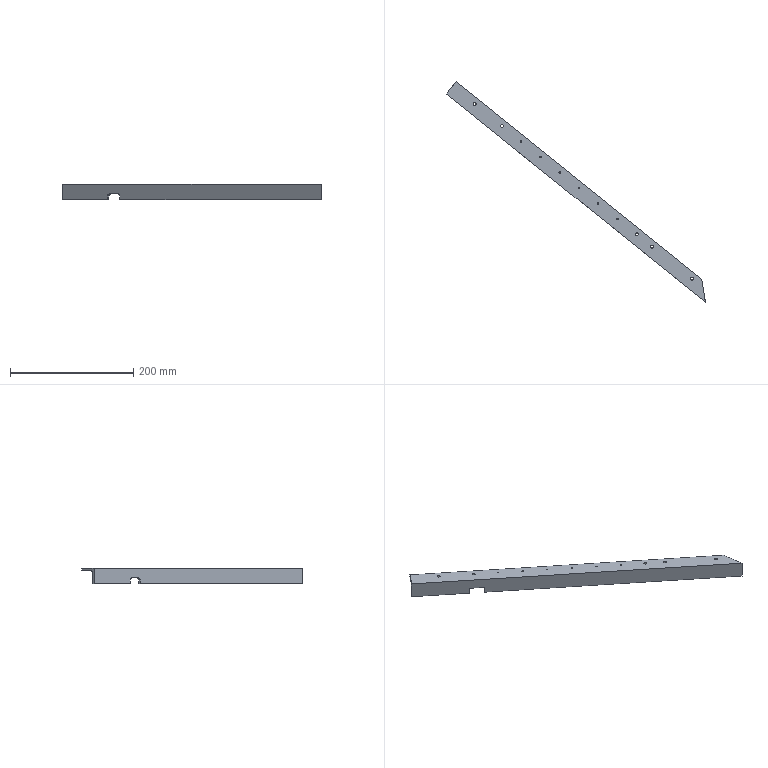Part | NX | features MG0301 nose pivot 24(right) 2 | 1 solid | 26 faces | box 419.376 x 356.955 x 25.4 mm | volume 81586 mm3 | cylinder 14 | plane 12 | commonest cylinder face diameters 2.4 x6 4.763 x5 6.35 x2 9.525 x1
STEP:
#1=CARTESIAN_POINT('',(357.102,-185.029,113.315));
#2=VERTEX_POINT('',#1);
#3=CARTESIAN_POINT('',(357.102,-185.029,106.965));
#4=VERTEX_POINT('',#3);
#5=CARTESIAN_POINT('',(357.102,-185.029,113.315));
#6=DIRECTION('',(0.,0.,-1.));
#7=VECTOR('',#6,1000.);
#8=LINE('',#5,#7);
#9=EDGE_CURVE('',#2,#4,#8,.T.);
#10=ORIENTED_EDGE('',*,*,#9,.F.);
#11=CARTESIAN_POINT('',(359.577,-187.018,116.49));
#12=VERTEX_POINT('',#11);
#13=CARTESIAN_POINT('',(359.577,-187.018,113.315));
#14=DIRECTION('',(-0.6266,-0.7794,0.));
#15=DIRECTION('',(0.7794,-0.6266,0.));
#16=AXIS2_PLACEMENT_3D('',#13,#14,#15);
#17=CIRCLE('',#16,3.175);
#18=EDGE_CURVE('',#12,#2,#17,.T.);
#19=ORIENTED_EDGE('',*,*,#18,.F.);
#20=CARTESIAN_POINT('',(374.424,-198.955,116.49));
#21=VERTEX_POINT('',#20);
#22=CARTESIAN_POINT('',(374.424,-198.955,116.49));
#23=DIRECTION('',(-0.7794,0.6266,0.));
#24=VECTOR('',#23,1000.);
#25=LINE('',#22,#24);
#26=EDGE_CURVE('',#21,#12,#25,.T.);
#27=ORIENTED_EDGE('',*,*,#26,.F.);
#28=CARTESIAN_POINT('',(376.898,-200.944,113.315));
#29=VERTEX_POINT('',#28);
#30=CARTESIAN_POINT('',(374.424,-198.955,113.315));
#31=DIRECTION('',(-0.6266,-0.7794,0.));
#32=DIRECTION('',(0.7794,-0.6266,0.));
#33=AXIS2_PLACEMENT_3D('',#30,#31,#32);
#34=CIRCLE('',#33,3.175);
#35=EDGE_CURVE('',#29,#21,#34,.T.);
#36=ORIENTED_EDGE('',*,*,#35,.F.);
#37=CARTESIAN_POINT('',(376.898,-200.944,106.965));
#38=VERTEX_POINT('',#37);
#39=CARTESIAN_POINT('',(376.898,-200.944,106.965));
#40=DIRECTION('',(0.,0.,1.));
#41=VECTOR('',#40,1000.);
#42=LINE('',#39,#41);
#43=EDGE_CURVE('',#38,#29,#42,.T.);
#44=ORIENTED_EDGE('',*,*,#43,.F.);
#45=CARTESIAN_POINT('',(703.42,-463.453,106.965));
#46=VERTEX_POINT('',#45);
#47=CARTESIAN_POINT('',(284.044,-126.294,106.965));
#48=DIRECTION('',(0.7794,-0.6266,0.));
#49=VECTOR('',#48,1000.);
#50=LINE('',#47,#49);
#51=EDGE_CURVE('',#46,#38,#50,.F.);
#52=ORIENTED_EDGE('',*,*,#51,.F.);
#53=CARTESIAN_POINT('',(703.42,-463.453,132.365));
#54=VERTEX_POINT('',#53);
#55=CARTESIAN_POINT('',(703.42,-463.453,132.365));
#56=DIRECTION('',(0.,0.,1.));
#57=VECTOR('',#56,1000.);
#58=LINE('',#55,#57);
#59=EDGE_CURVE('',#54,#46,#58,.F.);
#60=ORIENTED_EDGE('',*,*,#59,.F.);
#61=CARTESIAN_POINT('',(284.044,-126.294,132.365));
#62=VERTEX_POINT('',#61);
#63=CARTESIAN_POINT('',(284.044,-126.294,132.365));
#64=DIRECTION('',(0.7794,-0.6266,0.));
#65=VECTOR('',#64,1000.);
#66=LINE('',#63,#65);
#67=EDGE_CURVE('',#54,#62,#66,.F.);
#68=ORIENTED_EDGE('',*,*,#67,.T.);
#69=CARTESIAN_POINT('',(284.044,-126.294,106.965));
#70=VERTEX_POINT('',#69);
#71=CARTESIAN_POINT('',(284.044,-126.294,132.365));
#72=DIRECTION('',(0.,0.,1.));
#73=VECTOR('',#72,1000.);
#74=LINE('',#71,#73);
#75=EDGE_CURVE('',#62,#70,#74,.F.);
#76=ORIENTED_EDGE('',*,*,#75,.T.);
#77=CARTESIAN_POINT('',(284.044,-126.294,106.965));
#78=DIRECTION('',(0.7794,-0.6266,0.));
#79=VECTOR('',#78,1000.);
#80=LINE('',#77,#79);
#81=EDGE_CURVE('',#4,#70,#80,.F.);
#82=ORIENTED_EDGE('',*,*,#81,.F.);
#83=EDGE_LOOP('',(#10,#19,#27,#36,#44,#52,#60,#68,#76,#82));
#84=FACE_BOUND('',#83,.T.);
#85=CARTESIAN_POINT('',(284.044,-126.294,132.365));
#86=DIRECTION('',(0.6266,0.7794,0.));
#87=DIRECTION('',(-0.7794,0.6266,0.));
#88=AXIS2_PLACEMENT_3D('',#85,#86,#87);
#89=PLANE('',#88);
#90=ADVANCED_FACE('',(#84),#89,.F.);
#91=CARTESIAN_POINT('',(378.888,-198.469,106.965));
#92=VERTEX_POINT('',#91);
#93=CARTESIAN_POINT('',(383.164,-193.15,106.965));
#94=DIRECTION('',(-0.6266,-0.7794,0.));
#95=VECTOR('',#94,1000.);
#96=LINE('',#93,#95);
#97=EDGE_CURVE('',#92,#38,#96,.T.);
#98=ORIENTED_EDGE('',*,*,#97,.F.);
#99=CARTESIAN_POINT('',(702.681,-458.785,106.965));
#100=VERTEX_POINT('',#99);
#101=CARTESIAN_POINT('',(286.034,-123.819,106.965));
#102=DIRECTION('',(0.7794,-0.6266,0.));
#103=VECTOR('',#102,1000.);
#104=LINE('',#101,#103);
#105=EDGE_CURVE('',#100,#92,#104,.F.);
#106=ORIENTED_EDGE('',*,*,#105,.F.);
#107=CARTESIAN_POINT('',(641.063,-69.747,106.965));
#108=DIRECTION('',(0.1564,-0.9877,0.));
#109=VECTOR('',#108,1000.);
#110=LINE('',#107,#109);
#111=EDGE_CURVE('',#46,#100,#110,.F.);
#112=ORIENTED_EDGE('',*,*,#111,.F.);
#113=ORIENTED_EDGE('',*,*,#51,.T.);
#114=EDGE_LOOP('',(#98,#106,#112,#113));
#115=FACE_BOUND('',#114,.T.);
#116=CARTESIAN_POINT('',(284.044,-126.294,106.965));
#117=DIRECTION('',(0.,0.,1.));
#118=DIRECTION('',(0.9931,0.1177,0.));
#119=AXIS2_PLACEMENT_3D('',#116,#117,#118);
#120=PLANE('',#119);
#121=ADVANCED_FACE('',(#115),#120,.F.);
#122=CARTESIAN_POINT('',(437.141,-229.007,129.19));
#123=VERTEX_POINT('',#122);
#124=CARTESIAN_POINT('',(436.205,-228.255,129.19));
#125=DIRECTION('',(0.,0.,1.));
#126=DIRECTION('',(0.7794,-0.6266,0.));
#127=AXIS2_PLACEMENT_3D('',#124,#125,#126);
#128=CIRCLE('',#127,1.2);
#129=EDGE_CURVE('',#123,#123,#128,.F.);
#130=ORIENTED_EDGE('',*,*,#129,.F.);
#131=EDGE_LOOP('',(#130));
#132=FACE_BOUND('',#131,.T.);
#133=CARTESIAN_POINT('',(499.49,-279.133,129.19));
#134=VERTEX_POINT('',#133);
#135=CARTESIAN_POINT('',(498.554,-278.381,129.19));
#136=DIRECTION('',(0.,0.,1.));
#137=DIRECTION('',(0.7794,-0.6266,0.));
#138=AXIS2_PLACEMENT_3D('',#135,#136,#137);
#139=CIRCLE('',#138,1.2);
#140=EDGE_CURVE('',#134,#134,#139,.F.);
#141=ORIENTED_EDGE('',*,*,#140,.F.);
#142=EDGE_LOOP('',(#141));
#143=FACE_BOUND('',#142,.T.);
#144=CARTESIAN_POINT('',(561.839,-329.259,129.19));
#145=VERTEX_POINT('',#144);
#146=CARTESIAN_POINT('',(560.903,-328.507,129.19));
#147=DIRECTION('',(0.,0.,1.));
#148=DIRECTION('',(0.7794,-0.6266,0.));
#149=AXIS2_PLACEMENT_3D('',#146,#147,#148);
#150=CIRCLE('',#149,1.2);
#151=EDGE_CURVE('',#145,#145,#150,.F.);
#152=ORIENTED_EDGE('',*,*,#151,.F.);
#153=EDGE_LOOP('',(#152));
#154=FACE_BOUND('',#153,.T.);
#155=CARTESIAN_POINT('',(376.221,-177.849,129.19));
#156=VERTEX_POINT('',#155);
#157=CARTESIAN_POINT('',(373.856,-178.129,129.19));
#158=DIRECTION('',(0.,0.,1.));
#159=DIRECTION('',(0.9931,0.1177,0.));
#160=AXIS2_PLACEMENT_3D('',#157,#158,#159);
#161=CIRCLE('',#160,2.381);
#162=EDGE_CURVE('',#156,#156,#161,.F.);
#163=ORIENTED_EDGE('',*,*,#162,.F.);
#164=EDGE_LOOP('',(#163));
#165=FACE_BOUND('',#164,.T.);
#166=CARTESIAN_POINT('',(331.889,-142.208,129.19));
#167=VERTEX_POINT('',#166);
#168=CARTESIAN_POINT('',(329.524,-142.488,129.19));
#169=DIRECTION('',(0.,0.,1.));
#170=DIRECTION('',(0.9931,0.1177,0.));
#171=AXIS2_PLACEMENT_3D('',#168,#169,#170);
#172=CIRCLE('',#171,2.381);
#173=EDGE_CURVE('',#167,#167,#172,.F.);
#174=ORIENTED_EDGE('',*,*,#173,.F.);
#175=EDGE_LOOP('',(#174));
#176=FACE_BOUND('',#175,.T.);
#177=CARTESIAN_POINT('',(619.193,-373.188,129.19));
#178=VERTEX_POINT('',#177);
#179=CARTESIAN_POINT('',(616.829,-373.468,129.19));
#180=DIRECTION('',(0.,0.,1.));
#181=DIRECTION('',(0.9931,0.1177,0.));
#182=AXIS2_PLACEMENT_3D('',#179,#180,#181);
#183=CIRCLE('',#182,2.381);
#184=EDGE_CURVE('',#178,#178,#183,.F.);
#185=ORIENTED_EDGE('',*,*,#184,.F.);
#186=EDGE_LOOP('',(#185));
#187=FACE_BOUND('',#186,.T.);
#188=CARTESIAN_POINT('',(594.449,-353.294,129.19));
#189=VERTEX_POINT('',#188);
#190=CARTESIAN_POINT('',(592.084,-353.574,129.19));
#191=DIRECTION('',(0.,0.,1.));
#192=DIRECTION('',(0.9931,0.1177,0.));
#193=AXIS2_PLACEMENT_3D('',#190,#191,#192);
#194=CIRCLE('',#193,2.381);
#195=EDGE_CURVE('',#189,#189,#194,.F.);
#196=ORIENTED_EDGE('',*,*,#195,.F.);
#197=EDGE_LOOP('',(#196));
#198=FACE_BOUND('',#197,.T.);
#199=CARTESIAN_POINT('',(683.67,-425.024,129.19));
#200=VERTEX_POINT('',#199);
#201=CARTESIAN_POINT('',(681.305,-425.304,129.19));
#202=DIRECTION('',(0.,0.,1.));
#203=DIRECTION('',(0.9931,0.1177,0.));
#204=AXIS2_PLACEMENT_3D('',#201,#202,#203);
#205=CIRCLE('',#204,2.381);
#206=EDGE_CURVE('',#200,#200,#205,.F.);
#207=ORIENTED_EDGE('',*,*,#206,.F.);
#208=EDGE_LOOP('',(#207));
#209=FACE_BOUND('',#208,.T.);
#210=CARTESIAN_POINT('',(697.505,-426.107,129.19));
#211=VERTEX_POINT('',#210);
#212=CARTESIAN_POINT('',(299.959,-106.498,129.19));
#213=VERTEX_POINT('',#212);
#214=CARTESIAN_POINT('',(299.959,-106.498,129.19));
#215=DIRECTION('',(0.7794,-0.6266,0.));
#216=VECTOR('',#215,1000.);
#217=LINE('',#214,#216);
#218=EDGE_CURVE('',#211,#213,#217,.F.);
#219=ORIENTED_EDGE('',*,*,#218,.F.);
#220=CARTESIAN_POINT('',(701.572,-451.782,129.19));
#221=VERTEX_POINT('',#220);
#222=CARTESIAN_POINT('',(638.394,-52.895,129.19));
#223=DIRECTION('',(0.1564,-0.9877,0.));
#224=VECTOR('',#223,1000.);
#225=LINE('',#222,#224);
#226=EDGE_CURVE('',#221,#211,#225,.F.);
#227=ORIENTED_EDGE('',*,*,#226,.F.);
#228=CARTESIAN_POINT('',(289.018,-120.107,129.19));
#229=VERTEX_POINT('',#228);
#230=CARTESIAN_POINT('',(289.018,-120.107,129.19));
#231=DIRECTION('',(0.7794,-0.6266,0.));
#232=VECTOR('',#231,1000.);
#233=LINE('',#230,#232);
#234=EDGE_CURVE('',#221,#229,#233,.F.);
#235=ORIENTED_EDGE('',*,*,#234,.T.);
#236=CARTESIAN_POINT('',(299.959,-106.498,129.19));
#237=DIRECTION('',(-0.6266,-0.7794,0.));
#238=VECTOR('',#237,1000.);
#239=LINE('',#236,#238);
#240=EDGE_CURVE('',#229,#213,#239,.F.);
#241=ORIENTED_EDGE('',*,*,#240,.T.);
#242=EDGE_LOOP('',(#219,#227,#235,#241));
#243=FACE_BOUND('',#242,.T.);
#244=CARTESIAN_POINT('',(530.664,-304.196,129.19));
#245=VERTEX_POINT('',#244);
#246=CARTESIAN_POINT('',(529.729,-303.444,129.19));
#247=DIRECTION('',(0.,0.,1.));
#248=DIRECTION('',(0.7794,-0.6266,0.));
#249=AXIS2_PLACEMENT_3D('',#246,#247,#248);
#250=CIRCLE('',#249,1.2);
#251=EDGE_CURVE('',#245,#245,#250,.F.);
#252=ORIENTED_EDGE('',*,*,#251,.F.);
#253=EDGE_LOOP('',(#252));
#254=FACE_BOUND('',#253,.T.);
#255=CARTESIAN_POINT('',(468.315,-254.07,129.19));
#256=VERTEX_POINT('',#255);
#257=CARTESIAN_POINT('',(467.38,-253.318,129.19));
#258=DIRECTION('',(0.,0.,1.));
#259=DIRECTION('',(0.7794,-0.6266,0.));
#260=AXIS2_PLACEMENT_3D('',#257,#258,#259);
#261=CIRCLE('',#260,1.2);
#262=EDGE_CURVE('',#256,#256,#261,.F.);
#263=ORIENTED_EDGE('',*,*,#262,.F.);
#264=EDGE_LOOP('',(#263));
#265=FACE_BOUND('',#264,.T.);
#266=CARTESIAN_POINT('',(405.966,-203.944,129.19));
#267=VERTEX_POINT('',#266);
#268=CARTESIAN_POINT('',(405.031,-203.192,129.19));
#269=DIRECTION('',(0.,0.,1.));
#270=DIRECTION('',(0.7794,-0.6266,0.));
#271=AXIS2_PLACEMENT_3D('',#268,#269,#270);
#272=CIRCLE('',#271,1.2);
#273=EDGE_CURVE('',#267,#267,#272,.F.);
#274=ORIENTED_EDGE('',*,*,#273,.F.);
#275=EDGE_LOOP('',(#274));
#276=FACE_BOUND('',#275,.T.);
#277=CARTESIAN_POINT('',(299.959,-106.498,129.19));
#278=DIRECTION('',(0.,0.,1.));
#279=DIRECTION('',(0.9931,0.1177,0.));
#280=AXIS2_PLACEMENT_3D('',#277,#278,#279);
#281=PLANE('',#280);
#282=ADVANCED_FACE('',(#132,#143,#154,#165,#176,#187,#198,#209,#243,#254,#265,#276),#281,.F.);
#283=CARTESIAN_POINT('',(406.222,-203.051,132.365));
#284=VERTEX_POINT('',#283);
#285=CARTESIAN_POINT('',(405.031,-203.192,132.365));
#286=DIRECTION('',(0.,0.,1.));
#287=DIRECTION('',(0.9931,0.1177,0.));
#288=AXIS2_PLACEMENT_3D('',#285,#286,#287);
#289=CIRCLE('',#288,1.2);
#290=EDGE_CURVE('',#284,#284,#289,.F.);
#291=ORIENTED_EDGE('',*,*,#290,.T.);
#292=EDGE_LOOP('',(#291));
#293=FACE_BOUND('',#292,.T.);
#294=CARTESIAN_POINT('',(437.397,-228.114,132.365));
#295=VERTEX_POINT('',#294);
#296=CARTESIAN_POINT('',(436.205,-228.255,132.365));
#297=DIRECTION('',(0.,0.,1.));
#298=DIRECTION('',(0.9931,0.1177,0.));
#299=AXIS2_PLACEMENT_3D('',#296,#297,#298);
#300=CIRCLE('',#299,1.2);
#301=EDGE_CURVE('',#295,#295,#300,.F.);
#302=ORIENTED_EDGE('',*,*,#301,.T.);
#303=EDGE_LOOP('',(#302));
#304=FACE_BOUND('',#303,.T.);
#305=CARTESIAN_POINT('',(468.572,-253.177,132.365));
#306=VERTEX_POINT('',#305);
#307=CARTESIAN_POINT('',(467.38,-253.318,132.365));
#308=DIRECTION('',(0.,0.,1.));
#309=DIRECTION('',(0.9931,0.1177,0.));
#310=AXIS2_PLACEMENT_3D('',#307,#308,#309);
#311=CIRCLE('',#310,1.2);
#312=EDGE_CURVE('',#306,#306,#311,.F.);
#313=ORIENTED_EDGE('',*,*,#312,.T.);
#314=EDGE_LOOP('',(#313));
#315=FACE_BOUND('',#314,.T.);
#316=CARTESIAN_POINT('',(499.746,-278.24,132.365));
#317=VERTEX_POINT('',#316);
#318=CARTESIAN_POINT('',(498.554,-278.381,132.365));
#319=DIRECTION('',(0.,0.,1.));
#320=DIRECTION('',(0.9931,0.1177,0.));
#321=AXIS2_PLACEMENT_3D('',#318,#319,#320);
#322=CIRCLE('',#321,1.2);
#323=EDGE_CURVE('',#317,#317,#322,.F.);
#324=ORIENTED_EDGE('',*,*,#323,.T.);
#325=EDGE_LOOP('',(#324));
#326=FACE_BOUND('',#325,.T.);
#327=CARTESIAN_POINT('',(530.921,-303.303,132.365));
#328=VERTEX_POINT('',#327);
#329=CARTESIAN_POINT('',(529.729,-303.444,132.365));
#330=DIRECTION('',(0.,0.,1.));
#331=DIRECTION('',(0.9931,0.1177,0.));
#332=AXIS2_PLACEMENT_3D('',#329,#330,#331);
#333=CIRCLE('',#332,1.2);
#334=EDGE_CURVE('',#328,#328,#333,.F.);
#335=ORIENTED_EDGE('',*,*,#334,.T.);
#336=EDGE_LOOP('',(#335));
#337=FACE_BOUND('',#336,.T.);
#338=CARTESIAN_POINT('',(562.095,-328.365,132.365));
#339=VERTEX_POINT('',#338);
#340=CARTESIAN_POINT('',(560.903,-328.507,132.365));
#341=DIRECTION('',(0.,0.,1.));
#342=DIRECTION('',(0.9931,0.1177,0.));
#343=AXIS2_PLACEMENT_3D('',#340,#341,#342);
#344=CIRCLE('',#343,1.2);
#345=EDGE_CURVE('',#339,#339,#344,.F.);
#346=ORIENTED_EDGE('',*,*,#345,.T.);
#347=EDGE_LOOP('',(#346));
#348=FACE_BOUND('',#347,.T.);
#349=CARTESIAN_POINT('',(376.221,-177.849,132.365));
#350=VERTEX_POINT('',#349);
#351=CARTESIAN_POINT('',(373.856,-178.129,132.365));
#352=DIRECTION('',(0.,0.,1.));
#353=DIRECTION('',(0.9931,0.1177,0.));
#354=AXIS2_PLACEMENT_3D('',#351,#352,#353);
#355=CIRCLE('',#354,2.381);
#356=EDGE_CURVE('',#350,#350,#355,.F.);
#357=ORIENTED_EDGE('',*,*,#356,.T.);
#358=EDGE_LOOP('',(#357));
#359=FACE_BOUND('',#358,.T.);
#360=CARTESIAN_POINT('',(331.889,-142.208,132.365));
#361=VERTEX_POINT('',#360);
#362=CARTESIAN_POINT('',(329.524,-142.488,132.365));
#363=DIRECTION('',(0.,0.,1.));
#364=DIRECTION('',(0.9931,0.1177,0.));
#365=AXIS2_PLACEMENT_3D('',#362,#363,#364);
#366=CIRCLE('',#365,2.381);
#367=EDGE_CURVE('',#361,#361,#366,.F.);
#368=ORIENTED_EDGE('',*,*,#367,.T.);
#369=EDGE_LOOP('',(#368));
#370=FACE_BOUND('',#369,.T.);
#371=CARTESIAN_POINT('',(619.193,-373.188,132.365));
#372=VERTEX_POINT('',#371);
#373=CARTESIAN_POINT('',(616.829,-373.468,132.365));
#374=DIRECTION('',(0.,0.,1.));
#375=DIRECTION('',(0.9931,0.1177,0.));
#376=AXIS2_PLACEMENT_3D('',#373,#374,#375);
#377=CIRCLE('',#376,2.381);
#378=EDGE_CURVE('',#372,#372,#377,.F.);
#379=ORIENTED_EDGE('',*,*,#378,.T.);
#380=EDGE_LOOP('',(#379));
#381=FACE_BOUND('',#380,.T.);
#382=CARTESIAN_POINT('',(594.449,-353.294,132.365));
#383=VERTEX_POINT('',#382);
#384=CARTESIAN_POINT('',(592.084,-353.574,132.365));
#385=DIRECTION('',(0.,0.,1.));
#386=DIRECTION('',(0.9931,0.1177,0.));
#387=AXIS2_PLACEMENT_3D('',#384,#385,#386);
#388=CIRCLE('',#387,2.381);
#389=EDGE_CURVE('',#383,#383,#388,.F.);
#390=ORIENTED_EDGE('',*,*,#389,.T.);
#391=EDGE_LOOP('',(#390));
#392=FACE_BOUND('',#391,.T.);
#393=CARTESIAN_POINT('',(683.67,-425.024,132.365));
#394=VERTEX_POINT('',#393);
#395=CARTESIAN_POINT('',(681.305,-425.304,132.365));
#396=DIRECTION('',(0.,0.,1.));
#397=DIRECTION('',(0.9931,0.1177,0.));
#398=AXIS2_PLACEMENT_3D('',#395,#396,#397);
#399=CIRCLE('',#398,2.381);
#400=EDGE_CURVE('',#394,#394,#399,.F.);
#401=ORIENTED_EDGE('',*,*,#400,.T.);
#402=EDGE_LOOP('',(#401));
#403=FACE_BOUND('',#402,.T.);
#404=ORIENTED_EDGE('',*,*,#67,.F.);
#405=CARTESIAN_POINT('',(697.505,-426.107,132.365));
#406=VERTEX_POINT('',#405);
#407=CARTESIAN_POINT('',(641.063,-69.747,132.365));
#408=DIRECTION('',(-0.1564,0.9877,0.));
#409=VECTOR('',#408,1000.);
#410=LINE('',#407,#409);
#411=EDGE_CURVE('',#406,#54,#410,.F.);
#412=ORIENTED_EDGE('',*,*,#411,.F.);
#413=CARTESIAN_POINT('',(299.959,-106.498,132.365));
#414=VERTEX_POINT('',#413);
#415=CARTESIAN_POINT('',(299.959,-106.498,132.365));
#416=DIRECTION('',(0.7794,-0.6266,0.));
#417=VECTOR('',#416,1000.);
#418=LINE('',#415,#417);
#419=EDGE_CURVE('',#406,#414,#418,.F.);
#420=ORIENTED_EDGE('',*,*,#419,.T.);
#421=CARTESIAN_POINT('',(284.044,-126.294,132.365));
#422=DIRECTION('',(0.6266,0.7794,0.));
#423=VECTOR('',#422,1000.);
#424=LINE('',#421,#423);
#425=EDGE_CURVE('',#414,#62,#424,.F.);
#426=ORIENTED_EDGE('',*,*,#425,.T.);
#427=EDGE_LOOP('',(#404,#412,#420,#426));
#428=FACE_BOUND('',#427,.T.);
#429=CARTESIAN_POINT('',(284.044,-126.294,132.365));
#430=DIRECTION('',(0.,0.,-1.));
#431=DIRECTION('',(-0.9931,-0.1177,0.));
#432=AXIS2_PLACEMENT_3D('',#429,#430,#431);
#433=PLANE('',#432);
#434=ADVANCED_FACE('',(#293,#304,#315,#326,#337,#348,#359,#370,#381,#392,#403,#428),#433,.F.);
#435=ORIENTED_EDGE('',*,*,#419,.F.);
#436=CARTESIAN_POINT('',(697.505,-426.107,132.365));
#437=DIRECTION('',(0.,0.,-1.));
#438=VECTOR('',#437,1000.);
#439=LINE('',#436,#438);
#440=EDGE_CURVE('',#211,#406,#439,.F.);
#441=ORIENTED_EDGE('',*,*,#440,.F.);
#442=ORIENTED_EDGE('',*,*,#218,.T.);
#443=CARTESIAN_POINT('',(299.959,-106.498,132.365));
#444=DIRECTION('',(0.,0.,-1.));
#445=VECTOR('',#444,1000.);
#446=LINE('',#443,#445);
#447=EDGE_CURVE('',#213,#414,#446,.F.);
#448=ORIENTED_EDGE('',*,*,#447,.T.);
#449=EDGE_LOOP('',(#435,#441,#442,#448));
#450=FACE_BOUND('',#449,.T.);
#451=CARTESIAN_POINT('',(299.959,-106.498,132.365));
#452=DIRECTION('',(-0.6266,-0.7794,0.));
#453=DIRECTION('',(0.7794,-0.6266,0.));
#454=AXIS2_PLACEMENT_3D('',#451,#452,#453);
#455=PLANE('',#454);
#456=ADVANCED_FACE('',(#450),#455,.F.);
#457=ORIENTED_EDGE('',*,*,#234,.F.);
#458=CARTESIAN_POINT('',(702.681,-458.785,124.427));
#459=VERTEX_POINT('',#458);
#460=CARTESIAN_POINT('',(701.572,-451.782,124.427));
#461=DIRECTION('',(-0.9877,-0.1564,0.));
#462=DIRECTION('',(0.1564,-0.9877,0.));
#463=AXIS2_PLACEMENT_3D('',#460,#461,#462);
#464=ELLIPSE('',#463,7.09,4.763);
#465=EDGE_CURVE('',#459,#221,#464,.T.);
#466=ORIENTED_EDGE('',*,*,#465,.F.);
#467=CARTESIAN_POINT('',(286.034,-123.819,124.427));
#468=VERTEX_POINT('',#467);
#469=CARTESIAN_POINT('',(286.034,-123.819,124.427));
#470=DIRECTION('',(0.7794,-0.6266,0.));
#471=VECTOR('',#470,1000.);
#472=LINE('',#469,#471);
#473=EDGE_CURVE('',#459,#468,#472,.F.);
#474=ORIENTED_EDGE('',*,*,#473,.T.);
#475=CARTESIAN_POINT('',(289.018,-120.107,124.427));
#476=DIRECTION('',(0.7794,-0.6266,0.));
#477=DIRECTION('',(-0.6266,-0.7794,0.));
#478=AXIS2_PLACEMENT_3D('',#475,#476,#477);
#479=CIRCLE('',#478,4.763);
#480=EDGE_CURVE('',#468,#229,#479,.F.);
#481=ORIENTED_EDGE('',*,*,#480,.T.);
#482=EDGE_LOOP('',(#457,#466,#474,#481));
#483=FACE_BOUND('',#482,.T.);
#484=CARTESIAN_POINT('',(289.018,-120.107,124.427));
#485=DIRECTION('',(0.7794,-0.6266,0.));
#486=DIRECTION('',(0.6266,0.7794,0.));
#487=AXIS2_PLACEMENT_3D('',#484,#485,#486);
#488=CYLINDRICAL_SURFACE('',#487,4.763);
#489=ADVANCED_FACE('',(#483),#488,.F.);
#490=CARTESIAN_POINT('',(361.566,-184.544,116.49));
#491=VERTEX_POINT('',#490);
#492=CARTESIAN_POINT('',(359.092,-182.555,113.315));
#493=VERTEX_POINT('',#492);
#494=CARTESIAN_POINT('',(361.566,-184.544,113.315));
#495=DIRECTION('',(-0.6266,-0.7794,0.));
#496=DIRECTION('',(0.7794,-0.6266,0.));
#497=AXIS2_PLACEMENT_3D('',#494,#495,#496);
#498=CIRCLE('',#497,3.175);
#499=EDGE_CURVE('',#491,#493,#498,.T.);
#500=ORIENTED_EDGE('',*,*,#499,.T.);
#501=CARTESIAN_POINT('',(359.092,-182.555,106.965));
#502=VERTEX_POINT('',#501);
#503=CARTESIAN_POINT('',(359.092,-182.555,106.965));
#504=DIRECTION('',(0.,0.,-1.));
#505=VECTOR('',#504,1000.);
#506=LINE('',#503,#505);
#507=EDGE_CURVE('',#493,#502,#506,.T.);
#508=ORIENTED_EDGE('',*,*,#507,.T.);
#509=CARTESIAN_POINT('',(286.034,-123.819,106.965));
#510=VERTEX_POINT('',#509);
#511=CARTESIAN_POINT('',(286.034,-123.819,106.965));
#512=DIRECTION('',(0.7794,-0.6266,0.));
#513=VECTOR('',#512,1000.);
#514=LINE('',#511,#513);
#515=EDGE_CURVE('',#502,#510,#514,.F.);
#516=ORIENTED_EDGE('',*,*,#515,.T.);
#517=CARTESIAN_POINT('',(286.034,-123.819,106.965));
#518=DIRECTION('',(0.,0.,-1.));
#519=VECTOR('',#518,1000.);
#520=LINE('',#517,#519);
#521=EDGE_CURVE('',#510,#468,#520,.F.);
#522=ORIENTED_EDGE('',*,*,#521,.T.);
#523=ORIENTED_EDGE('',*,*,#473,.F.);
#524=CARTESIAN_POINT('',(702.681,-458.785,106.965));
#525=DIRECTION('',(0.,0.,-1.));
#526=VECTOR('',#525,1000.);
#527=LINE('',#524,#526);
#528=EDGE_CURVE('',#100,#459,#527,.F.);
#529=ORIENTED_EDGE('',*,*,#528,.F.);
#530=ORIENTED_EDGE('',*,*,#105,.T.);
#531=CARTESIAN_POINT('',(378.888,-198.469,113.315));
#532=VERTEX_POINT('',#531);
#533=CARTESIAN_POINT('',(378.888,-198.469,106.965));
#534=DIRECTION('',(0.,0.,1.));
#535=VECTOR('',#534,1000.);
#536=LINE('',#533,#535);
#537=EDGE_CURVE('',#92,#532,#536,.T.);
#538=ORIENTED_EDGE('',*,*,#537,.T.);
#539=CARTESIAN_POINT('',(376.413,-196.48,116.49));
#540=VERTEX_POINT('',#539);
#541=CARTESIAN_POINT('',(376.413,-196.48,113.315));
#542=DIRECTION('',(-0.6266,-0.7794,0.));
#543=DIRECTION('',(0.7794,-0.6266,0.));
#544=AXIS2_PLACEMENT_3D('',#541,#542,#543);
#545=CIRCLE('',#544,3.175);
#546=EDGE_CURVE('',#532,#540,#545,.T.);
#547=ORIENTED_EDGE('',*,*,#546,.T.);
#548=CARTESIAN_POINT('',(286.034,-123.819,116.49));
#549=DIRECTION('',(-0.7794,0.6266,0.));
#550=VECTOR('',#549,1000.);
#551=LINE('',#548,#550);
#552=EDGE_CURVE('',#540,#491,#551,.T.);
#553=ORIENTED_EDGE('',*,*,#552,.T.);
#554=EDGE_LOOP('',(#500,#508,#516,#522,#523,#529,#530,#538,#547,#553));
#555=FACE_BOUND('',#554,.T.);
#556=CARTESIAN_POINT('',(286.034,-123.819,106.965));
#557=DIRECTION('',(-0.6266,-0.7794,0.));
#558=DIRECTION('',(0.7794,-0.6266,0.));
#559=AXIS2_PLACEMENT_3D('',#556,#557,#558);
#560=PLANE('',#559);
#561=ADVANCED_FACE('',(#555),#560,.F.);
#562=ORIENTED_EDGE('',*,*,#515,.F.);
#563=CARTESIAN_POINT('',(363.368,-177.235,106.965));
#564=DIRECTION('',(-0.6266,-0.7794,0.));
#565=VECTOR('',#564,1000.);
#566=LINE('',#563,#565);
#567=EDGE_CURVE('',#502,#4,#566,.T.);
#568=ORIENTED_EDGE('',*,*,#567,.T.);
#569=ORIENTED_EDGE('',*,*,#81,.T.);
#570=CARTESIAN_POINT('',(284.044,-126.294,106.965));
#571=DIRECTION('',(-0.6266,-0.7794,0.));
#572=VECTOR('',#571,1000.);
#573=LINE('',#570,#572);
#574=EDGE_CURVE('',#70,#510,#573,.F.);
#575=ORIENTED_EDGE('',*,*,#574,.T.);
#576=EDGE_LOOP('',(#562,#568,#569,#575));
#577=FACE_BOUND('',#576,.T.);
#578=CARTESIAN_POINT('',(284.044,-126.294,106.965));
#579=DIRECTION('',(0.,0.,1.));
#580=DIRECTION('',(0.9931,0.1177,0.));
#581=AXIS2_PLACEMENT_3D('',#578,#579,#580);
#582=PLANE('',#581);
#583=ADVANCED_FACE('',(#577),#582,.F.);
#584=ORIENTED_EDGE('',*,*,#75,.F.);
#585=ORIENTED_EDGE('',*,*,#425,.F.);
#586=ORIENTED_EDGE('',*,*,#447,.F.);
#587=ORIENTED_EDGE('',*,*,#240,.F.);
#588=ORIENTED_EDGE('',*,*,#480,.F.);
#589=ORIENTED_EDGE('',*,*,#521,.F.);
#590=ORIENTED_EDGE('',*,*,#574,.F.);
#591=EDGE_LOOP('',(#584,#585,#586,#587,#588,#589,#590));
#592=FACE_BOUND('',#591,.T.);
#593=CARTESIAN_POINT('',(289.018,-120.107,124.427));
#594=DIRECTION('',(-0.7794,0.6266,0.));
#595=DIRECTION('',(-0.6266,-0.7794,0.));
#596=AXIS2_PLACEMENT_3D('',#593,#594,#595);
#597=PLANE('',#596);
#598=ADVANCED_FACE('',(#592),#597,.T.);
#599=ORIENTED_EDGE('',*,*,#411,.T.);
#600=ORIENTED_EDGE('',*,*,#59,.T.);
#601=ORIENTED_EDGE('',*,*,#111,.T.);
#602=ORIENTED_EDGE('',*,*,#528,.T.);
#603=ORIENTED_EDGE('',*,*,#465,.T.);
#604=ORIENTED_EDGE('',*,*,#226,.T.);
#605=ORIENTED_EDGE('',*,*,#440,.T.);
#606=EDGE_LOOP('',(#599,#600,#601,#602,#603,#604,#605));
#607=FACE_BOUND('',#606,.T.);
#608=CARTESIAN_POINT('',(703.42,-463.453,988.442));
#609=DIRECTION('',(-0.9877,-0.1564,0.));
#610=DIRECTION('',(0.1564,-0.9877,0.));
#611=AXIS2_PLACEMENT_3D('',#608,#609,#610);
#612=PLANE('',#611);
#613=ADVANCED_FACE('',(#607),#612,.F.);
#614=ORIENTED_EDGE('',*,*,#400,.F.);
#615=EDGE_LOOP('',(#614));
#616=FACE_BOUND('',#615,.T.);
#617=ORIENTED_EDGE('',*,*,#206,.T.);
#618=EDGE_LOOP('',(#617));
#619=FACE_BOUND('',#618,.T.);
#620=CARTESIAN_POINT('',(681.305,-425.304,68.865));
#621=DIRECTION('',(0.,0.,1.));
#622=DIRECTION('',(0.9931,0.1177,0.));
#623=AXIS2_PLACEMENT_3D('',#620,#621,#622);
#624=CYLINDRICAL_SURFACE('',#623,2.381);
#625=ADVANCED_FACE('',(#616,#619),#624,.F.);
#626=ORIENTED_EDGE('',*,*,#389,.F.);
#627=EDGE_LOOP('',(#626));
#628=FACE_BOUND('',#627,.T.);
#629=ORIENTED_EDGE('',*,*,#195,.T.);
#630=EDGE_LOOP('',(#629));
#631=FACE_BOUND('',#630,.T.);
#632=CARTESIAN_POINT('',(592.084,-353.574,68.865));
#633=DIRECTION('',(0.,0.,1.));
#634=DIRECTION('',(0.9931,0.1177,0.));
#635=AXIS2_PLACEMENT_3D('',#632,#633,#634);
#636=CYLINDRICAL_SURFACE('',#635,2.381);
#637=ADVANCED_FACE('',(#628,#631),#636,.F.);
#638=ORIENTED_EDGE('',*,*,#378,.F.);
#639=EDGE_LOOP('',(#638));
#640=FACE_BOUND('',#639,.T.);
#641=ORIENTED_EDGE('',*,*,#184,.T.);
#642=EDGE_LOOP('',(#641));
#643=FACE_BOUND('',#642,.T.);
#644=CARTESIAN_POINT('',(616.829,-373.468,68.865));
#645=DIRECTION('',(0.,0.,1.));
#646=DIRECTION('',(0.9931,0.1177,0.));
#647=AXIS2_PLACEMENT_3D('',#644,#645,#646);
#648=CYLINDRICAL_SURFACE('',#647,2.381);
#649=ADVANCED_FACE('',(#640,#643),#648,.F.);
#650=ORIENTED_EDGE('',*,*,#367,.F.);
#651=EDGE_LOOP('',(#650));
#652=FACE_BOUND('',#651,.T.);
#653=ORIENTED_EDGE('',*,*,#173,.T.);
#654=EDGE_LOOP('',(#653));
#655=FACE_BOUND('',#654,.T.);
#656=CARTESIAN_POINT('',(329.524,-142.488,68.865));
#657=DIRECTION('',(0.,0.,1.));
#658=DIRECTION('',(0.9931,0.1177,0.));
#659=AXIS2_PLACEMENT_3D('',#656,#657,#658);
#660=CYLINDRICAL_SURFACE('',#659,2.381);
#661=ADVANCED_FACE('',(#652,#655),#660,.F.);
#662=ORIENTED_EDGE('',*,*,#356,.F.);
#663=EDGE_LOOP('',(#662));
#664=FACE_BOUND('',#663,.T.);
#665=ORIENTED_EDGE('',*,*,#162,.T.);
#666=EDGE_LOOP('',(#665));
#667=FACE_BOUND('',#666,.T.);
#668=CARTESIAN_POINT('',(373.856,-178.129,68.865));
#669=DIRECTION('',(0.,0.,1.));
#670=DIRECTION('',(0.9931,0.1177,0.));
#671=AXIS2_PLACEMENT_3D('',#668,#669,#670);
#672=CYLINDRICAL_SURFACE('',#671,2.381);
#673=ADVANCED_FACE('',(#664,#667),#672,.F.);
#674=ORIENTED_EDGE('',*,*,#151,.T.);
#675=EDGE_LOOP('',(#674));
#676=FACE_BOUND('',#675,.T.);
#677=ORIENTED_EDGE('',*,*,#345,.F.);
#678=EDGE_LOOP('',(#677));
#679=FACE_BOUND('',#678,.T.);
#680=CARTESIAN_POINT('',(560.903,-328.507,139.19));
#681=DIRECTION('',(0.,0.,-1.));
#682=DIRECTION('',(0.9931,0.1177,0.));
#683=AXIS2_PLACEMENT_3D('',#680,#681,#682);
#684=CYLINDRICAL_SURFACE('',#683,1.2);
#685=ADVANCED_FACE('',(#676,#679),#684,.F.);
#686=ORIENTED_EDGE('',*,*,#251,.T.);
#687=EDGE_LOOP('',(#686));
#688=FACE_BOUND('',#687,.T.);
#689=ORIENTED_EDGE('',*,*,#334,.F.);
#690=EDGE_LOOP('',(#689));
#691=FACE_BOUND('',#690,.T.);
#692=CARTESIAN_POINT('',(529.729,-303.444,139.19));
#693=DIRECTION('',(0.,0.,-1.));
#694=DIRECTION('',(0.9931,0.1177,0.));
#695=AXIS2_PLACEMENT_3D('',#692,#693,#694);
#696=CYLINDRICAL_SURFACE('',#695,1.2);
#697=ADVANCED_FACE('',(#688,#691),#696,.F.);
#698=ORIENTED_EDGE('',*,*,#140,.T.);
#699=EDGE_LOOP('',(#698));
#700=FACE_BOUND('',#699,.T.);
#701=ORIENTED_EDGE('',*,*,#323,.F.);
#702=EDGE_LOOP('',(#701));
#703=FACE_BOUND('',#702,.T.);
#704=CARTESIAN_POINT('',(498.554,-278.381,139.19));
#705=DIRECTION('',(0.,0.,-1.));
#706=DIRECTION('',(0.9931,0.1177,0.));
#707=AXIS2_PLACEMENT_3D('',#704,#705,#706);
#708=CYLINDRICAL_SURFACE('',#707,1.2);
#709=ADVANCED_FACE('',(#700,#703),#708,.F.);
#710=ORIENTED_EDGE('',*,*,#262,.T.);
#711=EDGE_LOOP('',(#710));
#712=FACE_BOUND('',#711,.T.);
#713=ORIENTED_EDGE('',*,*,#312,.F.);
#714=EDGE_LOOP('',(#713));
#715=FACE_BOUND('',#714,.T.);
#716=CARTESIAN_POINT('',(467.38,-253.318,139.19));
#717=DIRECTION('',(0.,0.,-1.));
#718=DIRECTION('',(0.9931,0.1177,0.));
#719=AXIS2_PLACEMENT_3D('',#716,#717,#718);
#720=CYLINDRICAL_SURFACE('',#719,1.2);
#721=ADVANCED_FACE('',(#712,#715),#720,.F.);
#722=ORIENTED_EDGE('',*,*,#129,.T.);
#723=EDGE_LOOP('',(#722));
#724=FACE_BOUND('',#723,.T.);
#725=ORIENTED_EDGE('',*,*,#301,.F.);
#726=EDGE_LOOP('',(#725));
#727=FACE_BOUND('',#726,.T.);
#728=CARTESIAN_POINT('',(436.205,-228.255,139.19));
#729=DIRECTION('',(0.,0.,-1.));
#730=DIRECTION('',(0.9931,0.1177,0.));
#731=AXIS2_PLACEMENT_3D('',#728,#729,#730);
#732=CYLINDRICAL_SURFACE('',#731,1.2);
#733=ADVANCED_FACE('',(#724,#727),#732,.F.);
#734=ORIENTED_EDGE('',*,*,#273,.T.);
#735=EDGE_LOOP('',(#734));
#736=FACE_BOUND('',#735,.T.);
#737=ORIENTED_EDGE('',*,*,#290,.F.);
#738=EDGE_LOOP('',(#737));
#739=FACE_BOUND('',#738,.T.);
#740=CARTESIAN_POINT('',(405.031,-203.192,139.19));
#741=DIRECTION('',(0.,0.,-1.));
#742=DIRECTION('',(0.9931,0.1177,0.));
#743=AXIS2_PLACEMENT_3D('',#740,#741,#742);
#744=CYLINDRICAL_SURFACE('',#743,1.2);
#745=ADVANCED_FACE('',(#736,#739),#744,.F.);
#746=CARTESIAN_POINT('',(383.164,-193.15,113.315));
#747=DIRECTION('',(-0.6266,-0.7794,0.));
#748=VECTOR('',#747,1000.);
#749=LINE('',#746,#748);
#750=EDGE_CURVE('',#29,#532,#749,.F.);
#751=ORIENTED_EDGE('',*,*,#750,.F.);
#752=ORIENTED_EDGE('',*,*,#35,.T.);
#753=CARTESIAN_POINT('',(380.69,-191.161,116.49));
#754=DIRECTION('',(-0.6266,-0.7794,0.));
#755=VECTOR('',#754,1000.);
#756=LINE('',#753,#755);
#757=EDGE_CURVE('',#21,#540,#756,.F.);
#758=ORIENTED_EDGE('',*,*,#757,.T.);
#759=ORIENTED_EDGE('',*,*,#546,.F.);
#760=EDGE_LOOP('',(#751,#752,#758,#759));
#761=FACE_BOUND('',#760,.T.);
#762=CARTESIAN_POINT('',(380.69,-191.161,113.315));
#763=DIRECTION('',(-0.6266,-0.7794,0.));
#764=DIRECTION('',(0.7794,-0.6266,0.));
#765=AXIS2_PLACEMENT_3D('',#762,#763,#764);
#766=CYLINDRICAL_SURFACE('',#765,3.175);
#767=ADVANCED_FACE('',(#761),#766,.F.);
#768=ORIENTED_EDGE('',*,*,#757,.F.);
#769=ORIENTED_EDGE('',*,*,#26,.T.);
#770=CARTESIAN_POINT('',(365.843,-179.225,116.49));
#771=DIRECTION('',(-0.6266,-0.7794,0.));
#772=VECTOR('',#771,1000.);
#773=LINE('',#770,#772);
#774=EDGE_CURVE('',#12,#491,#773,.F.);
#775=ORIENTED_EDGE('',*,*,#774,.T.);
#776=ORIENTED_EDGE('',*,*,#552,.F.);
#777=EDGE_LOOP('',(#768,#769,#775,#776));
#778=FACE_BOUND('',#777,.T.);
#779=CARTESIAN_POINT('',(380.69,-191.161,116.49));
#780=DIRECTION('',(0.,0.,1.));
#781=DIRECTION('',(1.,0.,0.));
#782=AXIS2_PLACEMENT_3D('',#779,#780,#781);
#783=PLANE('',#782);
#784=ADVANCED_FACE('',(#778),#783,.F.);
#785=ORIENTED_EDGE('',*,*,#774,.F.);
#786=ORIENTED_EDGE('',*,*,#18,.T.);
#787=CARTESIAN_POINT('',(363.368,-177.235,113.315));
#788=DIRECTION('',(-0.6266,-0.7794,0.));
#789=VECTOR('',#788,1000.);
#790=LINE('',#787,#789);
#791=EDGE_CURVE('',#2,#493,#790,.F.);
#792=ORIENTED_EDGE('',*,*,#791,.T.);
#793=ORIENTED_EDGE('',*,*,#499,.F.);
#794=EDGE_LOOP('',(#785,#786,#792,#793));
#795=FACE_BOUND('',#794,.T.);
#796=CARTESIAN_POINT('',(365.843,-179.225,113.315));
#797=DIRECTION('',(-0.6266,-0.7794,0.));
#798=DIRECTION('',(0.7794,-0.6266,0.));
#799=AXIS2_PLACEMENT_3D('',#796,#797,#798);
#800=CYLINDRICAL_SURFACE('',#799,3.175);
#801=ADVANCED_FACE('',(#795),#800,.F.);
#802=ORIENTED_EDGE('',*,*,#791,.F.);
#803=ORIENTED_EDGE('',*,*,#9,.T.);
#804=ORIENTED_EDGE('',*,*,#567,.F.);
#805=ORIENTED_EDGE('',*,*,#507,.F.);
#806=EDGE_LOOP('',(#802,#803,#804,#805));
#807=FACE_BOUND('',#806,.T.);
#808=CARTESIAN_POINT('',(363.368,-177.235,113.315));
#809=DIRECTION('',(-0.7794,0.6266,0.));
#810=DIRECTION('',(-0.6266,-0.7794,0.));
#811=AXIS2_PLACEMENT_3D('',#808,#809,#810);
#812=PLANE('',#811);
#813=ADVANCED_FACE('',(#807),#812,.F.);
#814=ORIENTED_EDGE('',*,*,#97,.T.);
#815=ORIENTED_EDGE('',*,*,#43,.T.);
#816=ORIENTED_EDGE('',*,*,#750,.T.);
#817=ORIENTED_EDGE('',*,*,#537,.F.);
#818=EDGE_LOOP('',(#814,#815,#816,#817));
#819=FACE_BOUND('',#818,.T.);
#820=CARTESIAN_POINT('',(383.164,-193.15,106.965));
#821=DIRECTION('',(0.7794,-0.6266,0.));
#822=DIRECTION('',(0.6266,0.7794,0.));
#823=AXIS2_PLACEMENT_3D('',#820,#821,#822);
#824=PLANE('',#823);
#825=ADVANCED_FACE('',(#819),#824,.F.);
#826=CLOSED_SHELL('',(#90,#121,#282,#434,#456,#489,#561,#583,#598,#613,#625,#637,#649,#661,#673,#685,#697,#709,#721,#733,#745,#767,#784,#801,#813,#825));
#827=MANIFOLD_SOLID_BREP('',#826);
#828=(LENGTH_UNIT()NAMED_UNIT(*)SI_UNIT(.MILLI.,.METRE.));
#829=UNCERTAINTY_MEASURE_WITH_UNIT(LENGTH_MEASURE(0.00001),#828,'','');
#830=(NAMED_UNIT(*)PLANE_ANGLE_UNIT()SI_UNIT($,.RADIAN.));
#831=(NAMED_UNIT(*)SI_UNIT($,.STERADIAN.)SOLID_ANGLE_UNIT());
#832=(GEOMETRIC_REPRESENTATION_CONTEXT(3)GLOBAL_UNCERTAINTY_ASSIGNED_CONTEXT((#829))GLOBAL_UNIT_ASSIGNED_CONTEXT((#828,#830,#831))REPRESENTATION_CONTEXT('',''));
#833=ADVANCED_BREP_SHAPE_REPRESENTATION('',(#827),#832);